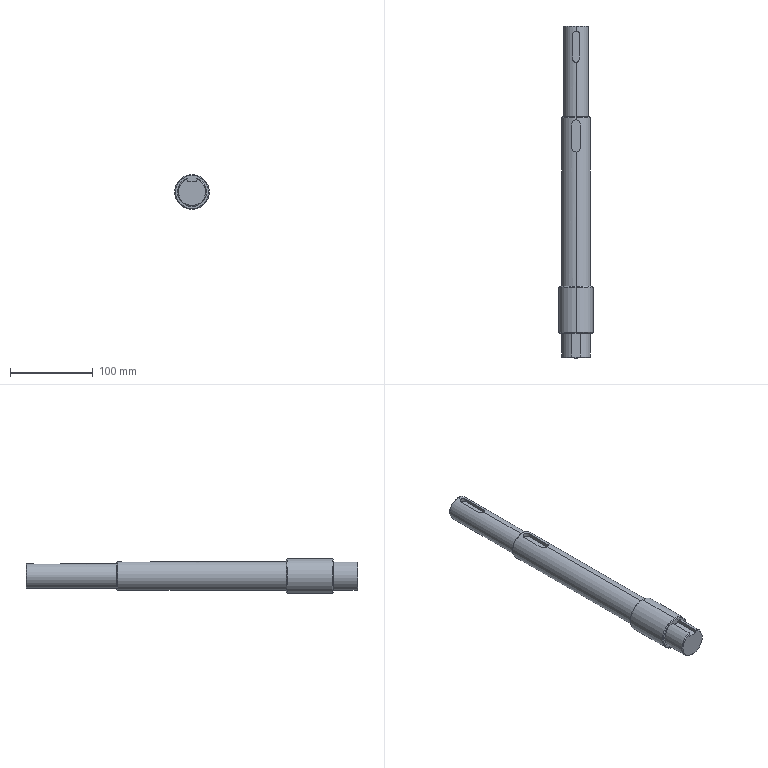Part | STEP file | PN_0017_default | 1 solid | 35 faces | box 42 x 401.5 x 42 mm | volume 377552 mm3 | plane 14 | cylinder 12 | cone 9 | commonest cylinder face diameters 35 x4 8 x2 10 x2 30 x2 42 x2